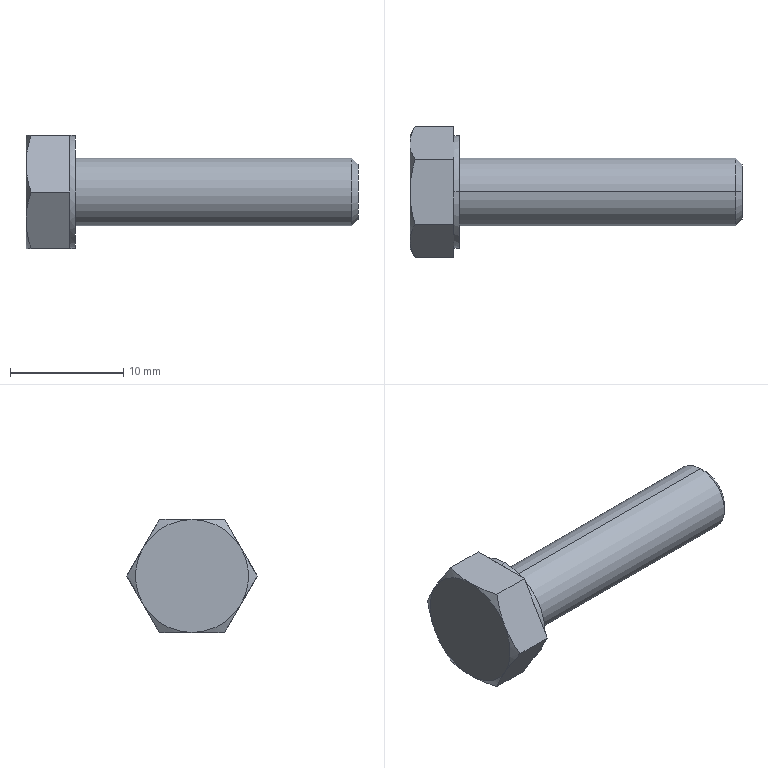Part | STEP file | hex screw gradec_iso(ISO 4018 - M6 x 25-WN) | 1 solid | 27 faces | box 29.375 x 11.547 x 10 mm | volume 1078 mm3 | plane 15 | cone 8 | cylinder 4 | commonest cylinder face diameters 6 x2 10 x2